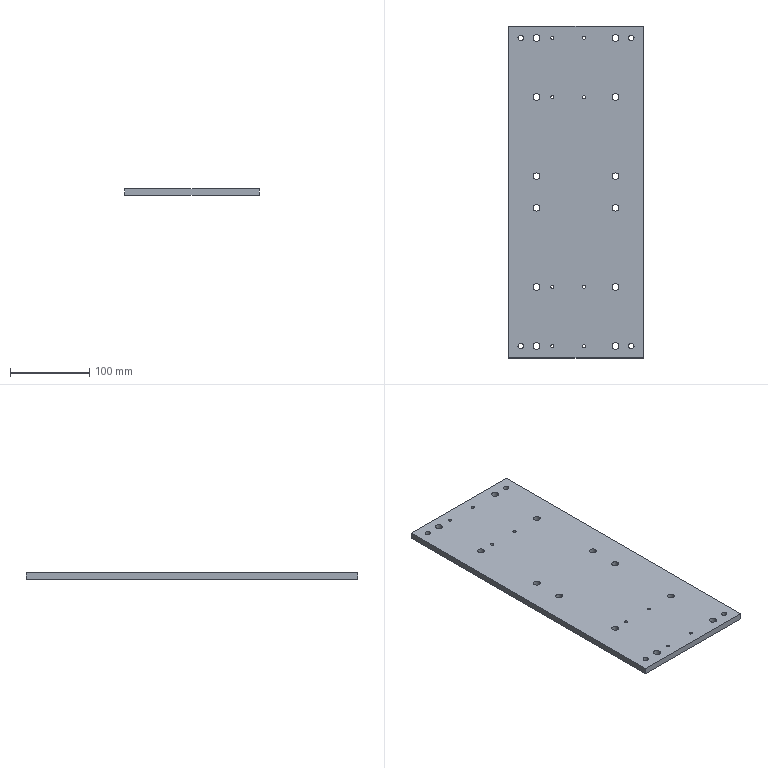Part | 1 solid | 54 faces | box 170 x 420 x 8 mm | volume 563657 mm3 | cylinder 48 | plane 6 | commonest cylinder face diameters 8.6 x24 4 x16 6.8 x8